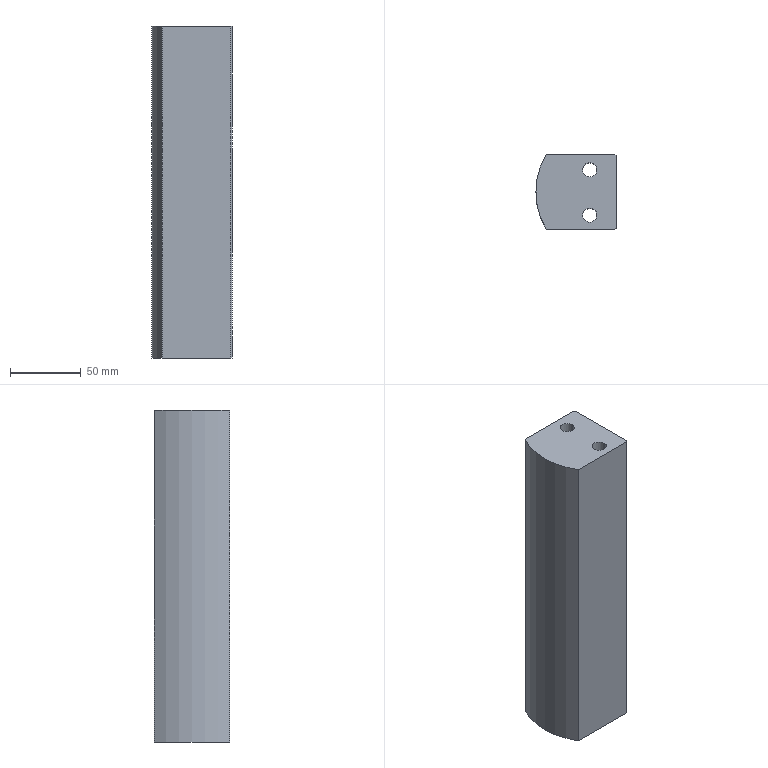Part | STEP file | 1 solid | 180 faces | box 56.5 x 53 x 234 mm | volume 627252 mm3 | cylinder 79 | cone 65 | plane 36 | commonest cylinder face diameters 4 x36 9 x36 10 x4 8 x2 105 x1